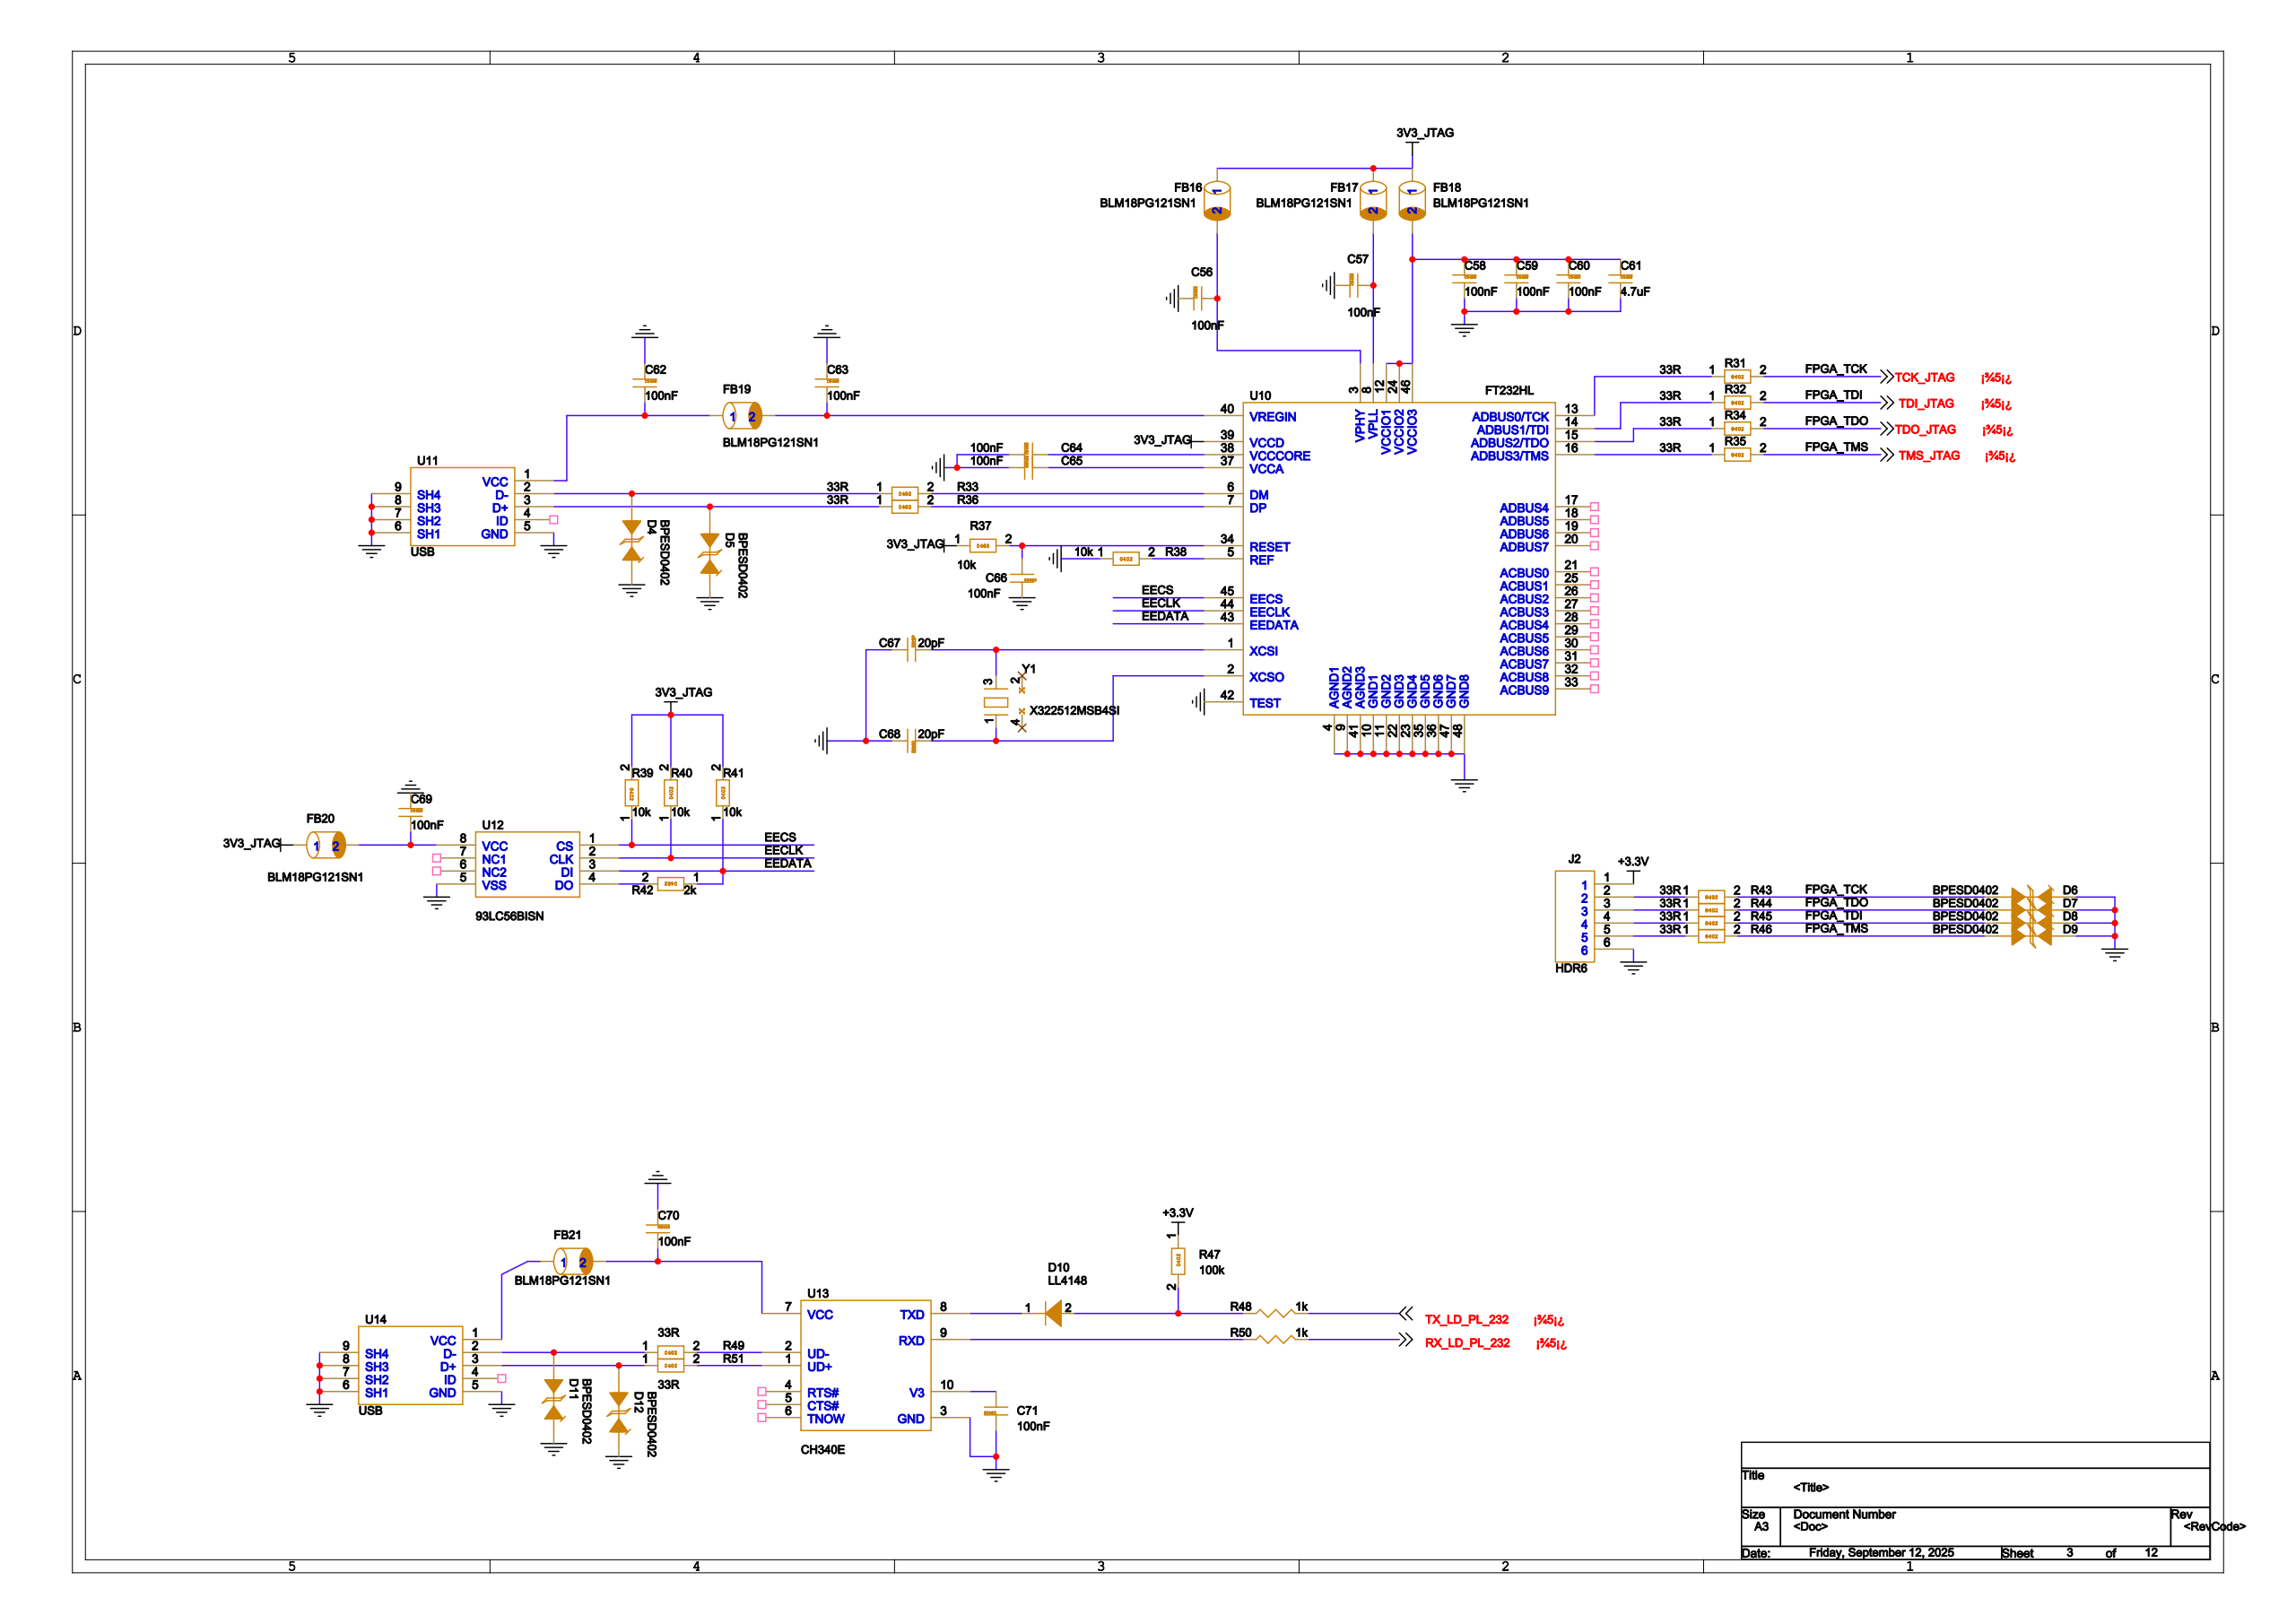Circuit board | Cadence Allegro | 528 parts | 530 nets | one sheet of the schematic
Parts on this sheet (reference | value | footprint):
C56 | 100nF | C0402
C57 | 100nF | C0402
C58 | 100nF | C0402
C59 | 100nF | C0402
C60 | 100nF | C0402
C61 | 4.7uF | C0603
C62 | 100nF | C0402
C63 | 100nF | C0402
C64 | 100nF | C0402
C65 | 100nF | C0402
C66 | 100nF | C0402
C67 | 20pF | C0402
C68 | 20pF | C0402
C69 | 100nF | C0402
C70 | 100nF | C0402
C71 | 100nF | C0402
D4 | BPESD0402 | C0402
D5 | BPESD0402 | C0402
D6 | BPESD0402 | C0402
D7 | BPESD0402 | C0402
D8 | BPESD0402 | C0402
D9 | BPESD0402 | C0402
D10 | LL4148 | SOD-80
D11 | BPESD0402 | C0402
D12 | BPESD0402 | C0402
FB16 | BLM18PG121SN1 | 0603
FB17 | BLM18PG121SN1 | 0603
FB18 | BLM18PG121SN1 | 0603
FB19 | BLM18PG121SN1 | 0603
FB20 | BLM18PG121SN1 | 0603
FB21 | BLM18PG121SN1 | 0603
J2 | HDR6 | HDR6-254MM
R31 | 33R | R0402
R32 | 33R | R0402
R33 | 33R | R0402
R34 | 33R | R0402
R35 | 33R | R0402
R36 | 33R | R0402
R37 | 10k | R0402
R38 | 10k | R0402
R39 | 10k | R0402
R40 | 10k | R0402
R41 | 10k | R0402
R42 | 2k | R0402
R43 | 33R | R0402
R44 | 33R | R0402
R45 | 33R | R0402
R46 | 33R | R0402
R47 | 100k | R0402
R48 | 1k | R0402
R49 | 33R | R0402
R50 | 1k | R0402
R51 | 33R | R0402
U10 | FT232HL | MOP10
U11 | USB | MICROUSB-AB
U12 | 93LC56BISN | SOIC8
U13 | CH340E | MSOP10
U14 | USB | MICROUSB-AB
Y1 | X322512MSB4SI | 3225-4
Nets of these parts (net: part-pin ...):
GND: C56-1 C57-1 C58-2 C59-2 C60-2 C61-2 C62-1 C63-1 C64-1 C65-1 C66-1 C67-2 C68-2 C69-1 C70-1 C71-1 D4-2 D5-2 D6-2 D7-2 D8-2 D9-2 D11-2 D12-2 J2-6 R38-1 U11-5 U11-6 U11-7 U11-8 U11-9 U12-5 U13-3 U14-5 U14-6 U14-7 U14-8 U14-9 U10-4 U10-9 U10-10 U10-11 U10-22 U10-23 U10-35 U10-36 U10-41 U10-42 U10-47 U10-48
N17763828: C68-1 Y1-1 U10-2
N17763822: C67-1 Y1-3 U10-1
+3.3V: J2-1 R47-1
N17778735: J2-2 R43-1
N17778738: J2-3 R44-1
N17778741: J2-4 R45-1
N17778744: J2-5 R46-1
N17763723: D5-1 R36-1 U11-3
N17763707: D4-1 R33-1 U11-2
N17763521: C62-2 FB19-1 U11-1
N18697864: D12-1 R51-1 U14-3
N18697848: D11-1 R49-1 U14-2
N18697743: FB21-1 U14-1
N17763366: C56-2 FB16-2 U10-3
N17763368: C57-2 FB17-2 U10-8
N17763370: C58-1 C59-1 C60-1 C61-1 FB18-2 U10-12 U10-24 U10-46
N17763531: C63-2 FB19-2 U10-40
N17763667: C64-2 U10-38
N17763693: C65-2 U10-37
N17763767: C66-2 R37-2 U10-34
N17763964: C69-2 FB20-2 U12-8
N18697733: C70-2 FB21-2 U13-7
N18697892: C71-2 U13-10
3V3_JTAG: FB16-1 FB17-1 FB18-1 FB20-1 R37-1 R39-2 R40-2 R41-2 U10-39
N17763501: R31-1 U10-13
TCK_JTAG: D6-1 R31-2 R43-2
N17763587: R32-1 U10-14
TDI_JTAG: D8-1 R32-2 R45-2
N17763719: R33-2 U10-6
N17763623: R34-1 U10-15
TDO_JTAG: D7-1 R34-2 R44-2
N17763669: R35-1 U10-16
TMS_JTAG: D9-1 R35-2 R46-2
N17763735: R36-2 U10-7
N18697860: R49-2 U13-2
N18697876: R51-2 U13-1
N17763785: R38-2 U10-5
EECS: R39-1 U12-1 U10-45
EECLK: R40-1 U12-2 U10-44
EEDATA: R41-1 R42-1 U12-3 U10-43
N18857403: R42-2 U12-4
N18697755: D10-2 R47-2 R48-2
TX_LD_PL_232: R48-1
RX_LD_PL_232: R50-1
N18697842: R50-2 U13-9
N18697798: D10-1 U13-8